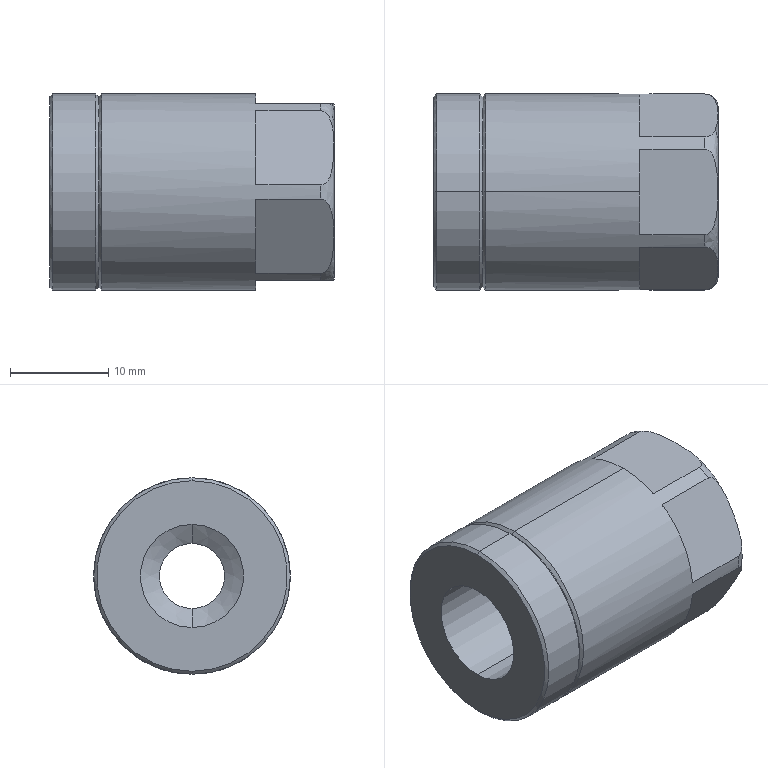Part | STEP file | _20MACJ15010A-Nut | 1 solid | 34 faces | box 29 x 20 x 20 mm | volume 7030 mm3 | plane 14 | cone 10 | cylinder 8 | spline 2 | commonest cylinder face diameters 20 x4 6.647 x2 10.5 x2
STEP:
#1=CARTESIAN_POINT('',(457.,0.,-8.6));
#2=VERTEX_POINT('',#1);
#3=CARTESIAN_POINT('',(457.,0.,8.6));
#4=VERTEX_POINT('',#3);
#5=CARTESIAN_POINT('',(457.,0.,-8.6));
#6=CARTESIAN_POINT('',(457.,-17.2,-8.6));
#7=CARTESIAN_POINT('',(457.,-17.2,8.6));
#8=CARTESIAN_POINT('',(457.,0.,8.6));
#9=(BOUNDED_CURVE()B_SPLINE_CURVE(3,(#5,#6,#7,#8),.UNSPECIFIED.,.F.,.F.)B_SPLINE_CURVE_WITH_KNOTS((4,4),(0.,0.5),.UNSPECIFIED.)CURVE()GEOMETRIC_REPRESENTATION_ITEM()RATIONAL_B_SPLINE_CURVE((1.,0.3333,0.3333,1.))REPRESENTATION_ITEM(''));
#10=EDGE_CURVE('',#2,#4,#9,.T.);
#11=ORIENTED_EDGE('',*,*,#10,.T.);
#12=CARTESIAN_POINT('',(456.942,0.,9.));
#13=VERTEX_POINT('',#12);
#14=CARTESIAN_POINT('',(455.6,0.,8.6));
#15=DIRECTION('',(0.,-1.,0.));
#16=DIRECTION('',(0.,0.,1.));
#17=AXIS2_PLACEMENT_3D('',#14,#15,#16);
#18=CIRCLE('',#17,1.4);
#19=EDGE_CURVE('',#4,#13,#18,.T.);
#20=ORIENTED_EDGE('',*,*,#19,.T.);
#21=CARTESIAN_POINT('',(455.6,-4.359,9.));
#22=VERTEX_POINT('',#21);
#23=CARTESIAN_POINT('',(455.6,-4.359,9.));
#24=CARTESIAN_POINT('',(455.704,-4.359,9.));
#25=CARTESIAN_POINT('',(455.805,-4.332,9.));
#26=CARTESIAN_POINT('',(455.989,-4.239,9.));
#27=CARTESIAN_POINT('',(456.071,-4.174,9.));
#28=CARTESIAN_POINT('',(456.214,-4.029,9.));
#29=CARTESIAN_POINT('',(456.277,-3.947,9.));
#30=CARTESIAN_POINT('',(456.388,-3.775,9.));
#31=CARTESIAN_POINT('',(456.435,-3.685,9.));
#32=CARTESIAN_POINT('',(456.563,-3.407,9.));
#33=CARTESIAN_POINT('',(456.628,-3.211,9.));
#34=CARTESIAN_POINT('',(456.731,-2.819,9.));
#35=CARTESIAN_POINT('',(456.769,-2.621,9.));
#36=CARTESIAN_POINT('',(456.863,-2.023,9.));
#37=CARTESIAN_POINT('',(456.895,-1.62,9.));
#38=CARTESIAN_POINT('',(456.934,-0.8093,9.));
#39=CARTESIAN_POINT('',(456.942,-0.4046,9.));
#40=CARTESIAN_POINT('',(456.942,0.,9.));
#41=B_SPLINE_CURVE_WITH_KNOTS('',3,(#23,#24,#25,#26,#27,#28,#29,#30,#31,#32,#33,#34,#35,#36,#37,#38,#39,#40),.UNSPECIFIED.,.F.,.F.,(4,2,2,2,2,2,2,2,4),(0.,0.0003068,0.0006136,0.0009205,0.001227,0.001841,0.002455,0.003682,0.004909),.UNSPECIFIED.);
#42=EDGE_CURVE('',#22,#13,#41,.T.);
#43=ORIENTED_EDGE('',*,*,#42,.F.);
#44=CARTESIAN_POINT('',(455.6,-5.615,8.275));
#45=VERTEX_POINT('',#44);
#46=CARTESIAN_POINT('',(455.6,0.,0.));
#47=DIRECTION('',(1.,0.,0.));
#48=DIRECTION('',(0.,0.,-1.));
#49=AXIS2_PLACEMENT_3D('',#46,#47,#48);
#50=CIRCLE('',#49,10.);
#51=EDGE_CURVE('',#22,#45,#50,.T.);
#52=ORIENTED_EDGE('',*,*,#51,.T.);
#53=CARTESIAN_POINT('',(455.6,-9.974,0.7251));
#54=VERTEX_POINT('',#53);
#55=CARTESIAN_POINT('',(455.6,-9.974,0.7251));
#56=CARTESIAN_POINT('',(455.704,-9.974,0.7251));
#57=CARTESIAN_POINT('',(455.805,-9.96,0.7487));
#58=CARTESIAN_POINT('',(455.989,-9.914,0.8289));
#59=CARTESIAN_POINT('',(456.071,-9.881,0.885));
#60=CARTESIAN_POINT('',(456.214,-9.809,1.011));
#61=CARTESIAN_POINT('',(456.277,-9.767,1.082));
#62=CARTESIAN_POINT('',(456.388,-9.681,1.231));
#63=CARTESIAN_POINT('',(456.436,-9.636,1.309));
#64=CARTESIAN_POINT('',(456.563,-9.498,1.549));
#65=CARTESIAN_POINT('',(456.628,-9.4,1.719));
#66=CARTESIAN_POINT('',(456.731,-9.204,2.059));
#67=CARTESIAN_POINT('',(456.77,-9.105,2.23));
#68=CARTESIAN_POINT('',(456.863,-8.806,2.748));
#69=CARTESIAN_POINT('',(456.895,-8.604,3.098));
#70=CARTESIAN_POINT('',(456.934,-8.198,3.8));
#71=CARTESIAN_POINT('',(456.942,-7.996,4.151));
#72=CARTESIAN_POINT('',(456.942,-7.591,4.851));
#73=CARTESIAN_POINT('',(456.934,-7.389,5.202));
#74=CARTESIAN_POINT('',(456.895,-6.985,5.902));
#75=CARTESIAN_POINT('',(456.863,-6.783,6.252));
#76=CARTESIAN_POINT('',(456.769,-6.481,6.774));
#77=CARTESIAN_POINT('',(456.729,-6.381,6.947));
#78=CARTESIAN_POINT('',(456.625,-6.184,7.288));
#79=CARTESIAN_POINT('',(456.561,-6.088,7.455));
#80=CARTESIAN_POINT('',(456.391,-5.904,7.774));
#81=CARTESIAN_POINT('',(456.285,-5.815,7.928));
#82=CARTESIAN_POINT('',(456.068,-5.706,8.117));
#83=CARTESIAN_POINT('',(455.988,-5.674,8.172));
#84=CARTESIAN_POINT('',(455.805,-5.628,8.251));
#85=CARTESIAN_POINT('',(455.703,-5.615,8.275));
#86=CARTESIAN_POINT('',(455.6,-5.615,8.275));
#87=B_SPLINE_CURVE_WITH_KNOTS('',3,(#55,#56,#57,#58,#59,#60,#61,#62,#63,#64,#65,#66,#67,#68,#69,#70,#71,#72,#73,#74,#75,#76,#77,#78,#79,#80,#81,#82,#83,#84,#85,#86),.UNSPECIFIED.,.F.,.F.,(4,2,2,2,2,2,2,2,2,2,2,2,2,2,2,4),(0.,0.0003069,0.0006138,0.0009207,0.001228,0.001841,0.002455,0.003683,0.00491,0.006138,0.007365,0.007979,0.008593,0.009207,0.009514,0.009821),.UNSPECIFIED.);
#88=EDGE_CURVE('',#54,#45,#87,.T.);
#89=ORIENTED_EDGE('',*,*,#88,.F.);
#90=CARTESIAN_POINT('',(455.6,-9.974,-0.7251));
#91=VERTEX_POINT('',#90);
#92=CARTESIAN_POINT('',(455.6,0.,0.));
#93=DIRECTION('',(1.,0.,0.));
#94=DIRECTION('',(0.,0.,-1.));
#95=AXIS2_PLACEMENT_3D('',#92,#93,#94);
#96=CIRCLE('',#95,10.);
#97=EDGE_CURVE('',#54,#91,#96,.T.);
#98=ORIENTED_EDGE('',*,*,#97,.T.);
#99=CARTESIAN_POINT('',(455.6,-5.615,-8.275));
#100=VERTEX_POINT('',#99);
#101=CARTESIAN_POINT('',(455.6,-5.615,-8.275));
#102=CARTESIAN_POINT('',(455.704,-5.615,-8.275));
#103=CARTESIAN_POINT('',(455.805,-5.628,-8.251));
#104=CARTESIAN_POINT('',(455.989,-5.675,-8.171));
#105=CARTESIAN_POINT('',(456.071,-5.707,-8.115));
#106=CARTESIAN_POINT('',(456.214,-5.78,-7.989));
#107=CARTESIAN_POINT('',(456.277,-5.821,-7.918));
#108=CARTESIAN_POINT('',(456.388,-5.907,-7.769));
#109=CARTESIAN_POINT('',(456.436,-5.952,-7.691));
#110=CARTESIAN_POINT('',(456.563,-6.091,-7.451));
#111=CARTESIAN_POINT('',(456.628,-6.189,-7.281));
#112=CARTESIAN_POINT('',(456.731,-6.385,-6.941));
#113=CARTESIAN_POINT('',(456.77,-6.484,-6.77));
#114=CARTESIAN_POINT('',(456.863,-6.783,-6.252));
#115=CARTESIAN_POINT('',(456.895,-6.985,-5.902));
#116=CARTESIAN_POINT('',(456.934,-7.39,-5.2));
#117=CARTESIAN_POINT('',(456.942,-7.592,-4.849));
#118=CARTESIAN_POINT('',(456.942,-7.997,-4.149));
#119=CARTESIAN_POINT('',(456.934,-8.199,-3.798));
#120=CARTESIAN_POINT('',(456.895,-8.603,-3.098));
#121=CARTESIAN_POINT('',(456.863,-8.806,-2.748));
#122=CARTESIAN_POINT('',(456.769,-9.107,-2.226));
#123=CARTESIAN_POINT('',(456.729,-9.207,-2.053));
#124=CARTESIAN_POINT('',(456.625,-9.404,-1.712));
#125=CARTESIAN_POINT('',(456.561,-9.501,-1.545));
#126=CARTESIAN_POINT('',(456.391,-9.684,-1.226));
#127=CARTESIAN_POINT('',(456.285,-9.773,-1.072));
#128=CARTESIAN_POINT('',(456.068,-9.883,-0.8826));
#129=CARTESIAN_POINT('',(455.988,-9.914,-0.8285));
#130=CARTESIAN_POINT('',(455.805,-9.96,-0.7485));
#131=CARTESIAN_POINT('',(455.703,-9.974,-0.7251));
#132=CARTESIAN_POINT('',(455.6,-9.974,-0.7251));
#133=B_SPLINE_CURVE_WITH_KNOTS('',3,(#101,#102,#103,#104,#105,#106,#107,#108,#109,#110,#111,#112,#113,#114,#115,#116,#117,#118,#119,#120,#121,#122,#123,#124,#125,#126,#127,#128,#129,#130,#131,#132),.UNSPECIFIED.,.F.,.F.,(4,2,2,2,2,2,2,2,2,2,2,2,2,2,2,4),(0.,0.0003069,0.0006138,0.0009207,0.001228,0.001841,0.002455,0.003683,0.00491,0.006138,0.007365,0.007979,0.008593,0.009207,0.009514,0.009821),.UNSPECIFIED.);
#134=EDGE_CURVE('',#100,#91,#133,.T.);
#135=ORIENTED_EDGE('',*,*,#134,.F.);
#136=CARTESIAN_POINT('',(455.6,-4.359,-9.));
#137=VERTEX_POINT('',#136);
#138=CARTESIAN_POINT('',(455.6,0.,0.));
#139=DIRECTION('',(1.,0.,0.));
#140=DIRECTION('',(0.,0.,-1.));
#141=AXIS2_PLACEMENT_3D('',#138,#139,#140);
#142=CIRCLE('',#141,10.);
#143=EDGE_CURVE('',#100,#137,#142,.T.);
#144=ORIENTED_EDGE('',*,*,#143,.T.);
#145=CARTESIAN_POINT('',(456.942,0.,-9.));
#146=VERTEX_POINT('',#145);
#147=CARTESIAN_POINT('',(456.942,0.,-9.));
#148=CARTESIAN_POINT('',(456.942,-0.4048,-9.));
#149=CARTESIAN_POINT('',(456.934,-0.8093,-9.));
#150=CARTESIAN_POINT('',(456.895,-1.618,-9.));
#151=CARTESIAN_POINT('',(456.863,-2.022,-9.));
#152=CARTESIAN_POINT('',(456.769,-2.626,-9.));
#153=CARTESIAN_POINT('',(456.729,-2.825,-9.));
#154=CARTESIAN_POINT('',(456.625,-3.219,-9.));
#155=CARTESIAN_POINT('',(456.561,-3.412,-9.));
#156=CARTESIAN_POINT('',(456.391,-3.78,-9.));
#157=CARTESIAN_POINT('',(456.285,-3.958,-9.));
#158=CARTESIAN_POINT('',(456.068,-4.177,-9.));
#159=CARTESIAN_POINT('',(455.988,-4.239,-9.));
#160=CARTESIAN_POINT('',(455.805,-4.332,-9.));
#161=CARTESIAN_POINT('',(455.703,-4.359,-9.));
#162=CARTESIAN_POINT('',(455.6,-4.359,-9.));
#163=B_SPLINE_CURVE_WITH_KNOTS('',3,(#147,#148,#149,#150,#151,#152,#153,#154,#155,#156,#157,#158,#159,#160,#161,#162),.UNSPECIFIED.,.F.,.F.,(4,2,2,2,2,2,2,4),(0.004909,0.006137,0.007365,0.007979,0.008593,0.009207,0.009514,0.009821),.UNSPECIFIED.);
#164=EDGE_CURVE('',#146,#137,#163,.T.);
#165=ORIENTED_EDGE('',*,*,#164,.F.);
#166=CARTESIAN_POINT('',(455.6,0.,-8.6));
#167=DIRECTION('',(0.,1.,0.));
#168=DIRECTION('',(0.,0.,-1.));
#169=AXIS2_PLACEMENT_3D('',#166,#167,#168);
#170=CIRCLE('',#169,1.4);
#171=EDGE_CURVE('',#2,#146,#170,.T.);
#172=ORIENTED_EDGE('',*,*,#171,.F.);
#173=EDGE_LOOP('',(#11,#20,#43,#52,#89,#98,#135,#144,#165,#172));
#174=FACE_OUTER_BOUND('',#173,.T.);
#175=CARTESIAN_POINT('',(457.,0.,8.6));
#176=CARTESIAN_POINT('',(457.,-17.2,8.6));
#177=CARTESIAN_POINT('',(457.,-17.2,-8.6));
#178=CARTESIAN_POINT('',(457.,0.,-8.6));
#179=CARTESIAN_POINT('',(457.,0.,9.42));
#180=CARTESIAN_POINT('',(457.,-18.84,9.42));
#181=CARTESIAN_POINT('',(457.,-18.84,-9.42));
#182=CARTESIAN_POINT('',(457.,0.,-9.42));
#183=CARTESIAN_POINT('',(456.42,0.,10.));
#184=CARTESIAN_POINT('',(456.42,-20.,10.));
#185=CARTESIAN_POINT('',(456.42,-20.,-10.));
#186=CARTESIAN_POINT('',(456.42,0.,-10.));
#187=CARTESIAN_POINT('',(455.6,0.,10.));
#188=CARTESIAN_POINT('',(455.6,-20.,10.));
#189=CARTESIAN_POINT('',(455.6,-20.,-10.));
#190=CARTESIAN_POINT('',(455.6,0.,-10.));
#191=(BOUNDED_SURFACE()B_SPLINE_SURFACE(3,3,((#175,#176,#177,#178),(#179,#180,#181,#182),(#183,#184,#185,#186),(#187,#188,#189,#190)),.UNSPECIFIED.,.F.,.F.,.T.)B_SPLINE_SURFACE_WITH_KNOTS((4,4),(4,4),(0.,1.),(0.,1.),.UNSPECIFIED.)GEOMETRIC_REPRESENTATION_ITEM()RATIONAL_B_SPLINE_SURFACE(((1.,0.3333,0.3333,1.),(0.8047,0.2682,0.2682,0.8047),(0.8047,0.2682,0.2682,0.8047),(1.,0.3333,0.3333,1.)))REPRESENTATION_ITEM('')SURFACE());
#192=ADVANCED_FACE('',(#174),#191,.T.);
#193=CARTESIAN_POINT('',(449.,4.359,-9.));
#194=VERTEX_POINT('',#193);
#195=CARTESIAN_POINT('',(449.,0.,-10.));
#196=VERTEX_POINT('',#195);
#197=CARTESIAN_POINT('',(449.,0.,0.));
#198=DIRECTION('',(-1.,0.,0.));
#199=DIRECTION('',(0.,0.,1.));
#200=AXIS2_PLACEMENT_3D('',#197,#198,#199);
#201=CIRCLE('',#200,10.);
#202=EDGE_CURVE('',#194,#196,#201,.T.);
#203=ORIENTED_EDGE('',*,*,#202,.T.);
#204=CARTESIAN_POINT('',(433.3,0.,-10.));
#205=VERTEX_POINT('',#204);
#206=CARTESIAN_POINT('',(457.,0.,-10.));
#207=DIRECTION('',(-1.,0.,0.));
#208=VECTOR('',#207,1000.);
#209=LINE('',#206,#208);
#210=EDGE_CURVE('',#196,#205,#209,.T.);
#211=ORIENTED_EDGE('',*,*,#210,.T.);
#212=CARTESIAN_POINT('',(433.3,0.,10.));
#213=VERTEX_POINT('',#212);
#214=CARTESIAN_POINT('',(433.3,0.,0.));
#215=DIRECTION('',(1.,0.,0.));
#216=DIRECTION('',(0.,0.,1.));
#217=AXIS2_PLACEMENT_3D('',#214,#215,#216);
#218=CIRCLE('',#217,10.);
#219=EDGE_CURVE('',#205,#213,#218,.T.);
#220=ORIENTED_EDGE('',*,*,#219,.T.);
#221=CARTESIAN_POINT('',(449.,0.,10.));
#222=VERTEX_POINT('',#221);
#223=CARTESIAN_POINT('',(457.,0.,10.));
#224=DIRECTION('',(-1.,0.,0.));
#225=VECTOR('',#224,1000.);
#226=LINE('',#223,#225);
#227=EDGE_CURVE('',#222,#213,#226,.T.);
#228=ORIENTED_EDGE('',*,*,#227,.F.);
#229=CARTESIAN_POINT('',(449.,4.359,9.));
#230=VERTEX_POINT('',#229);
#231=CARTESIAN_POINT('',(449.,0.,0.));
#232=DIRECTION('',(-1.,0.,0.));
#233=DIRECTION('',(0.,0.,1.));
#234=AXIS2_PLACEMENT_3D('',#231,#232,#233);
#235=CIRCLE('',#234,10.);
#236=EDGE_CURVE('',#222,#230,#235,.T.);
#237=ORIENTED_EDGE('',*,*,#236,.T.);
#238=CARTESIAN_POINT('',(455.6,4.359,9.));
#239=VERTEX_POINT('',#238);
#240=CARTESIAN_POINT('',(457.,4.359,9.));
#241=DIRECTION('',(1.,0.,0.));
#242=VECTOR('',#241,1000.);
#243=LINE('',#240,#242);
#244=EDGE_CURVE('',#230,#239,#243,.T.);
#245=ORIENTED_EDGE('',*,*,#244,.T.);
#246=CARTESIAN_POINT('',(455.6,5.615,8.275));
#247=VERTEX_POINT('',#246);
#248=CARTESIAN_POINT('',(455.6,0.,0.));
#249=DIRECTION('',(1.,0.,0.));
#250=DIRECTION('',(0.,0.,-1.));
#251=AXIS2_PLACEMENT_3D('',#248,#249,#250);
#252=CIRCLE('',#251,10.);
#253=EDGE_CURVE('',#247,#239,#252,.T.);
#254=ORIENTED_EDGE('',*,*,#253,.F.);
#255=CARTESIAN_POINT('',(449.,5.615,8.275));
#256=VERTEX_POINT('',#255);
#257=CARTESIAN_POINT('',(457.,5.615,8.275));
#258=DIRECTION('',(-1.,0.,0.));
#259=VECTOR('',#258,1000.);
#260=LINE('',#257,#259);
#261=EDGE_CURVE('',#247,#256,#260,.T.);
#262=ORIENTED_EDGE('',*,*,#261,.T.);
#263=CARTESIAN_POINT('',(449.,9.974,0.7251));
#264=VERTEX_POINT('',#263);
#265=CARTESIAN_POINT('',(449.,0.,0.));
#266=DIRECTION('',(-1.,0.,0.));
#267=DIRECTION('',(0.,0.,1.));
#268=AXIS2_PLACEMENT_3D('',#265,#266,#267);
#269=CIRCLE('',#268,10.);
#270=EDGE_CURVE('',#256,#264,#269,.T.);
#271=ORIENTED_EDGE('',*,*,#270,.T.);
#272=CARTESIAN_POINT('',(455.6,9.974,0.7251));
#273=VERTEX_POINT('',#272);
#274=CARTESIAN_POINT('',(457.,9.974,0.7251));
#275=DIRECTION('',(1.,0.,0.));
#276=VECTOR('',#275,1000.);
#277=LINE('',#274,#276);
#278=EDGE_CURVE('',#264,#273,#277,.T.);
#279=ORIENTED_EDGE('',*,*,#278,.T.);
#280=CARTESIAN_POINT('',(455.6,9.974,-0.7251));
#281=VERTEX_POINT('',#280);
#282=CARTESIAN_POINT('',(455.6,0.,0.));
#283=DIRECTION('',(1.,0.,0.));
#284=DIRECTION('',(0.,0.,-1.));
#285=AXIS2_PLACEMENT_3D('',#282,#283,#284);
#286=CIRCLE('',#285,10.);
#287=EDGE_CURVE('',#281,#273,#286,.T.);
#288=ORIENTED_EDGE('',*,*,#287,.F.);
#289=CARTESIAN_POINT('',(449.,9.974,-0.7251));
#290=VERTEX_POINT('',#289);
#291=CARTESIAN_POINT('',(457.,9.974,-0.7251));
#292=DIRECTION('',(-1.,0.,0.));
#293=VECTOR('',#292,1000.);
#294=LINE('',#291,#293);
#295=EDGE_CURVE('',#281,#290,#294,.T.);
#296=ORIENTED_EDGE('',*,*,#295,.T.);
#297=CARTESIAN_POINT('',(449.,5.615,-8.275));
#298=VERTEX_POINT('',#297);
#299=CARTESIAN_POINT('',(449.,0.,0.));
#300=DIRECTION('',(-1.,0.,0.));
#301=DIRECTION('',(0.,0.,1.));
#302=AXIS2_PLACEMENT_3D('',#299,#300,#301);
#303=CIRCLE('',#302,10.);
#304=EDGE_CURVE('',#290,#298,#303,.T.);
#305=ORIENTED_EDGE('',*,*,#304,.T.);
#306=CARTESIAN_POINT('',(455.6,5.615,-8.275));
#307=VERTEX_POINT('',#306);
#308=CARTESIAN_POINT('',(457.,5.615,-8.275));
#309=DIRECTION('',(1.,0.,0.));
#310=VECTOR('',#309,1000.);
#311=LINE('',#308,#310);
#312=EDGE_CURVE('',#298,#307,#311,.T.);
#313=ORIENTED_EDGE('',*,*,#312,.T.);
#314=CARTESIAN_POINT('',(455.6,4.359,-9.));
#315=VERTEX_POINT('',#314);
#316=CARTESIAN_POINT('',(455.6,0.,0.));
#317=DIRECTION('',(1.,0.,0.));
#318=DIRECTION('',(0.,0.,-1.));
#319=AXIS2_PLACEMENT_3D('',#316,#317,#318);
#320=CIRCLE('',#319,10.);
#321=EDGE_CURVE('',#315,#307,#320,.T.);
#322=ORIENTED_EDGE('',*,*,#321,.F.);
#323=CARTESIAN_POINT('',(457.,4.359,-9.));
#324=DIRECTION('',(-1.,0.,0.));
#325=VECTOR('',#324,1000.);
#326=LINE('',#323,#325);
#327=EDGE_CURVE('',#315,#194,#326,.T.);
#328=ORIENTED_EDGE('',*,*,#327,.T.);
#329=EDGE_LOOP('',(#203,#211,#220,#228,#237,#245,#254,#262,#271,#279,#288,#296,#305,#313,#322,#328));
#330=FACE_OUTER_BOUND('',#329,.T.);
#331=CARTESIAN_POINT('',(457.,0.,0.));
#332=DIRECTION('',(-1.,0.,0.));
#333=DIRECTION('',(0.,0.,1.));
#334=AXIS2_PLACEMENT_3D('',#331,#332,#333);
#335=CYLINDRICAL_SURFACE('',#334,10.);
#336=ADVANCED_FACE('',(#330),#335,.T.);
#337=CARTESIAN_POINT('',(433.,0.,-9.7));
#338=VERTEX_POINT('',#337);
#339=CARTESIAN_POINT('',(433.,0.,9.7));
#340=VERTEX_POINT('',#339);
#341=CARTESIAN_POINT('',(433.,0.,0.));
#342=DIRECTION('',(1.,0.,0.));
#343=DIRECTION('',(0.,0.,-1.));
#344=AXIS2_PLACEMENT_3D('',#341,#342,#343);
#345=CIRCLE('',#344,9.7);
#346=EDGE_CURVE('',#338,#340,#345,.T.);
#347=ORIENTED_EDGE('',*,*,#346,.T.);
#348=CARTESIAN_POINT('',(433.3,0.,10.));
#349=DIRECTION('',(0.7071,0.,0.7071));
#350=VECTOR('',#349,1000.);
#351=LINE('',#348,#350);
#352=EDGE_CURVE('',#340,#213,#351,.T.);
#353=ORIENTED_EDGE('',*,*,#352,.T.);
#354=ORIENTED_EDGE('',*,*,#219,.F.);
#355=CARTESIAN_POINT('',(433.3,0.,-10.));
#356=DIRECTION('',(0.7071,0.,-0.7071));
#357=VECTOR('',#356,1000.);
#358=LINE('',#355,#357);
#359=EDGE_CURVE('',#338,#205,#358,.T.);
#360=ORIENTED_EDGE('',*,*,#359,.F.);
#361=EDGE_LOOP('',(#347,#353,#354,#360));
#362=FACE_OUTER_BOUND('',#361,.T.);
#363=CARTESIAN_POINT('',(433.3,0.,0.));
#364=DIRECTION('',(1.,0.,0.));
#365=DIRECTION('',(0.,0.,-1.));
#366=AXIS2_PLACEMENT_3D('',#363,#364,#365);
#367=CONICAL_SURFACE('',#366,10.,0.7854);
#368=ADVANCED_FACE('',(#362),#367,.T.);
#369=ORIENTED_EDGE('',*,*,#346,.F.);
#370=CARTESIAN_POINT('',(432.7,0.,-10.));
#371=VERTEX_POINT('',#370);
#372=CARTESIAN_POINT('',(432.7,0.,-10.));
#373=DIRECTION('',(-0.7071,0.,-0.7071));
#374=VECTOR('',#373,1000.);
#375=LINE('',#372,#374);
#376=EDGE_CURVE('',#338,#371,#375,.T.);
#377=ORIENTED_EDGE('',*,*,#376,.T.);
#378=CARTESIAN_POINT('',(432.7,0.,10.));
#379=VERTEX_POINT('',#378);
#380=CARTESIAN_POINT('',(432.7,0.,0.));
#381=DIRECTION('',(1.,0.,0.));
#382=DIRECTION('',(0.,0.,1.));
#383=AXIS2_PLACEMENT_3D('',#380,#381,#382);
#384=CIRCLE('',#383,10.);
#385=EDGE_CURVE('',#371,#379,#384,.T.);
#386=ORIENTED_EDGE('',*,*,#385,.T.);
#387=CARTESIAN_POINT('',(432.7,0.,10.));
#388=DIRECTION('',(-0.7071,0.,0.7071));
#389=VECTOR('',#388,1000.);
#390=LINE('',#387,#389);
#391=EDGE_CURVE('',#340,#379,#390,.T.);
#392=ORIENTED_EDGE('',*,*,#391,.F.);
#393=EDGE_LOOP('',(#369,#377,#386,#392));
#394=FACE_OUTER_BOUND('',#393,.T.);
#395=CARTESIAN_POINT('',(432.7,0.,0.));
#396=DIRECTION('',(-1.,0.,0.));
#397=DIRECTION('',(0.,0.,1.));
#398=AXIS2_PLACEMENT_3D('',#395,#396,#397);
#399=CONICAL_SURFACE('',#398,10.,0.7854);
#400=ADVANCED_FACE('',(#394),#399,.T.);
#401=ORIENTED_EDGE('',*,*,#385,.F.);
#402=CARTESIAN_POINT('',(428.3,0.,-10.));
#403=VERTEX_POINT('',#402);
#404=CARTESIAN_POINT('',(457.,0.,-10.));
#405=DIRECTION('',(-1.,0.,0.));
#406=VECTOR('',#405,1000.);
#407=LINE('',#404,#406);
#408=EDGE_CURVE('',#371,#403,#407,.T.);
#409=ORIENTED_EDGE('',*,*,#408,.T.);
#410=CARTESIAN_POINT('',(428.3,0.,10.));
#411=VERTEX_POINT('',#410);
#412=CARTESIAN_POINT('',(428.3,0.,0.));
#413=DIRECTION('',(1.,0.,0.));
#414=DIRECTION('',(0.,0.,1.));
#415=AXIS2_PLACEMENT_3D('',#412,#413,#414);
#416=CIRCLE('',#415,10.);
#417=EDGE_CURVE('',#403,#411,#416,.T.);
#418=ORIENTED_EDGE('',*,*,#417,.T.);
#419=CARTESIAN_POINT('',(457.,0.,10.));
#420=DIRECTION('',(-1.,0.,0.));
#421=VECTOR('',#420,1000.);
#422=LINE('',#419,#421);
#423=EDGE_CURVE('',#379,#411,#422,.T.);
#424=ORIENTED_EDGE('',*,*,#423,.F.);
#425=EDGE_LOOP('',(#401,#409,#418,#424));
#426=FACE_OUTER_BOUND('',#425,.T.);
#427=CARTESIAN_POINT('',(457.,0.,0.));
#428=DIRECTION('',(-1.,0.,0.));
#429=DIRECTION('',(0.,0.,1.));
#430=AXIS2_PLACEMENT_3D('',#427,#428,#429);
#431=CYLINDRICAL_SURFACE('',#430,10.);
#432=ADVANCED_FACE('',(#426),#431,.T.);
#433=CARTESIAN_POINT('',(428.,0.,-9.7));
#434=VERTEX_POINT('',#433);
#435=CARTESIAN_POINT('',(428.,0.,9.7));
#436=VERTEX_POINT('',#435);
#437=CARTESIAN_POINT('',(428.,0.,0.));
#438=DIRECTION('',(1.,0.,0.));
#439=DIRECTION('',(0.,0.,-1.));
#440=AXIS2_PLACEMENT_3D('',#437,#438,#439);
#441=CIRCLE('',#440,9.7);
#442=EDGE_CURVE('',#434,#436,#441,.T.);
#443=ORIENTED_EDGE('',*,*,#442,.T.);
#444=CARTESIAN_POINT('',(428.3,0.,10.));
#445=DIRECTION('',(0.7071,0.,0.7071));
#446=VECTOR('',#445,1000.);
#447=LINE('',#444,#446);
#448=EDGE_CURVE('',#436,#411,#447,.T.);
#449=ORIENTED_EDGE('',*,*,#448,.T.);
#450=ORIENTED_EDGE('',*,*,#417,.F.);
#451=CARTESIAN_POINT('',(428.3,0.,-10.));
#452=DIRECTION('',(0.7071,0.,-0.7071));
#453=VECTOR('',#452,1000.);
#454=LINE('',#451,#453);
#455=EDGE_CURVE('',#434,#403,#454,.T.);
#456=ORIENTED_EDGE('',*,*,#455,.F.);
#457=EDGE_LOOP('',(#443,#449,#450,#456));
#458=FACE_OUTER_BOUND('',#457,.T.);
#459=CARTESIAN_POINT('',(428.3,0.,0.));
#460=DIRECTION('',(1.,0.,0.));
#461=DIRECTION('',(0.,0.,-1.));
#462=AXIS2_PLACEMENT_3D('',#459,#460,#461);
#463=CONICAL_SURFACE('',#462,10.,0.7854);
#464=ADVANCED_FACE('',(#458),#463,.T.);
#465=CARTESIAN_POINT('',(456.323,-3.323,0.));
#466=VERTEX_POINT('',#465);
#467=CARTESIAN_POINT('',(456.323,0.,-3.323));
#468=VERTEX_POINT('',#467);
#469=CARTESIAN_POINT('',(456.323,0.,0.));
#470=DIRECTION('',(1.,0.,0.));
#471=DIRECTION('',(0.,0.,-1.));
#472=AXIS2_PLACEMENT_3D('',#469,#470,#471);
#473=CIRCLE('',#472,3.323);
#474=EDGE_CURVE('',#466,#468,#473,.T.);
#475=ORIENTED_EDGE('',*,*,#474,.F.);
#476=CARTESIAN_POINT('',(457.,-4.,0.));
#477=VERTEX_POINT('',#476);
#478=CARTESIAN_POINT('',(457.,-4.,0.));
#479=DIRECTION('',(0.7071,-0.7071,0.));
#480=VECTOR('',#479,1000.);
#481=LINE('',#478,#480);
#482=EDGE_CURVE('',#466,#477,#481,.T.);
#483=ORIENTED_EDGE('',*,*,#482,.T.);
#484=CARTESIAN_POINT('',(457.,4.,0.));
#485=VERTEX_POINT('',#484);
#486=CARTESIAN_POINT('',(457.,0.,0.));
#487=DIRECTION('',(1.,0.,0.));
#488=DIRECTION('',(0.,1.,0.));
#489=AXIS2_PLACEMENT_3D('',#486,#487,#488);
#490=CIRCLE('',#489,4.);
#491=EDGE_CURVE('',#477,#485,#490,.T.);
#492=ORIENTED_EDGE('',*,*,#491,.T.);
#493=CARTESIAN_POINT('',(456.323,3.323,0.));
#494=VERTEX_POINT('',#493);
#495=CARTESIAN_POINT('',(457.,4.,0.));
#496=DIRECTION('',(0.7071,0.7071,0.));
#497=VECTOR('',#496,1000.);
#498=LINE('',#495,#497);
#499=EDGE_CURVE('',#494,#485,#498,.T.);
#500=ORIENTED_EDGE('',*,*,#499,.F.);
#501=CARTESIAN_POINT('',(456.323,0.,0.));
#502=DIRECTION('',(1.,0.,0.));
#503=DIRECTION('',(0.,0.,-1.));
#504=AXIS2_PLACEMENT_3D('',#501,#502,#503);
#505=CIRCLE('',#504,3.323);
#506=EDGE_CURVE('',#468,#494,#505,.T.);
#507=ORIENTED_EDGE('',*,*,#506,.F.);
#508=EDGE_LOOP('',(#475,#483,#492,#500,#507));
#509=FACE_OUTER_BOUND('',#508,.T.);
#510=CARTESIAN_POINT('',(457.,0.,0.));
#511=DIRECTION('',(1.,0.,0.));
#512=DIRECTION('',(0.,1.,0.));
#513=AXIS2_PLACEMENT_3D('',#510,#511,#512);
#514=CONICAL_SURFACE('',#513,4.,0.7854);
#515=ADVANCED_FACE('',(#509),#514,.F.);
#516=CARTESIAN_POINT('',(456.323,0.,3.323));
#517=VERTEX_POINT('',#516);
#518=CARTESIAN_POINT('',(456.323,0.,0.));
#519=DIRECTION('',(1.,0.,0.));
#520=DIRECTION('',(0.,0.,-1.));
#521=AXIS2_PLACEMENT_3D('',#518,#519,#520);
#522=CIRCLE('',#521,3.323);
#523=EDGE_CURVE('',#517,#466,#522,.T.);
#524=ORIENTED_EDGE('',*,*,#523,.T.);
#525=ORIENTED_EDGE('',*,*,#474,.T.);
#526=CARTESIAN_POINT('',(443.462,0.,-3.324));
#527=VERTEX_POINT('',#526);
#528=CARTESIAN_POINT('',(457.,0.,-3.324));
#529=DIRECTION('',(-1.,0.,0.));
#530=VECTOR('',#529,1000.);
#531=LINE('',#528,#530);
#532=EDGE_CURVE('',#468,#527,#531,.T.);
#533=ORIENTED_EDGE('',*,*,#532,.T.);
#534=CARTESIAN_POINT('',(443.462,0.,3.324));
#535=VERTEX_POINT('',#534);
#536=CARTESIAN_POINT('',(443.462,0.,0.));
#537=DIRECTION('',(1.,0.,0.));
#538=DIRECTION('',(0.,0.,1.));
#539=AXIS2_PLACEMENT_3D('',#536,#537,#538);
#540=CIRCLE('',#539,3.324);
#541=EDGE_CURVE('',#535,#527,#540,.T.);
#542=ORIENTED_EDGE('',*,*,#541,.F.);
#543=CARTESIAN_POINT('',(457.,0.,3.324));
#544=DIRECTION('',(-1.,0.,0.));
#545=VECTOR('',#544,1000.);
#546=LINE('',#543,#545);
#547=EDGE_CURVE('',#517,#535,#546,.T.);
#548=ORIENTED_EDGE('',*,*,#547,.F.);
#549=EDGE_LOOP('',(#524,#525,#533,#542,#548));
#550=FACE_OUTER_BOUND('',#549,.T.);
#551=CARTESIAN_POINT('',(457.,0.,0.));
#552=DIRECTION('',(-1.,0.,0.));
#553=DIRECTION('',(0.,0.,1.));
#554=AXIS2_PLACEMENT_3D('',#551,#552,#553);
#555=CYLINDRICAL_SURFACE('',#554,3.324);
#556=ADVANCED_FACE('',(#550),#555,.F.);
#557=CARTESIAN_POINT('',(442.35,0.,-5.25));
#558=VERTEX_POINT('',#557);
#559=CARTESIAN_POINT('',(442.35,0.,5.25));
#560=VERTEX_POINT('',#559);
#561=CARTESIAN_POINT('',(442.35,0.,0.));
#562=DIRECTION('',(-1.,0.,0.));
#563=DIRECTION('',(0.,0.,1.));
#564=AXIS2_PLACEMENT_3D('',#561,#562,#563);
#565=CIRCLE('',#564,5.25);
#566=EDGE_CURVE('',#558,#560,#565,.T.);
#567=ORIENTED_EDGE('',*,*,#566,.F.);
#568=CARTESIAN_POINT('',(428.,0.,-5.25));
#569=VERTEX_POINT('',#568);
#570=CARTESIAN_POINT('',(457.,0.,-5.25));
#571=DIRECTION('',(-1.,0.,0.));
#572=VECTOR('',#571,1000.);
#573=LINE('',#570,#572);
#574=EDGE_CURVE('',#558,#569,#573,.T.);
#575=ORIENTED_EDGE('',*,*,#574,.T.);
#576=CARTESIAN_POINT('',(428.,0.,5.25));
#577=VERTEX_POINT('',#576);
#578=CARTESIAN_POINT('',(428.,0.,0.));
#579=DIRECTION('',(-1.,0.,0.));
#580=DIRECTION('',(0.,0.,1.));
#581=AXIS2_PLACEMENT_3D('',#578,#579,#580);
#582=CIRCLE('',#581,5.25);
#583=EDGE_CURVE('',#569,#577,#582,.T.);
#584=ORIENTED_EDGE('',*,*,#583,.T.);
#585=CARTESIAN_POINT('',(457.,0.,5.25));
#586=DIRECTION('',(-1.,0.,0.));
#587=VECTOR('',#586,1000.);
#588=LINE('',#585,#587);
#589=EDGE_CURVE('',#560,#577,#588,.T.);
#590=ORIENTED_EDGE('',*,*,#589,.F.);
#591=EDGE_LOOP('',(#567,#575,#584,#590));
#592=FACE_OUTER_BOUND('',#591,.T.);
#593=CARTESIAN_POINT('',(457.,0.,0.));
#594=DIRECTION('',(-1.,0.,0.));
#595=DIRECTION('',(0.,0.,1.));
#596=AXIS2_PLACEMENT_3D('',#593,#594,#595);
#597=CYLINDRICAL_SURFACE('',#596,5.25);
#598=ADVANCED_FACE('',(#592),#597,.F.);
#599=ORIENTED_EDGE('',*,*,#541,.T.);
#600=CARTESIAN_POINT('',(442.35,0.,-5.25));
#601=DIRECTION('',(-0.5,0.,-0.866));
#602=VECTOR('',#601,1000.);
#603=LINE('',#600,#602);
#604=EDGE_CURVE('',#527,#558,#603,.T.);
#605=ORIENTED_EDGE('',*,*,#604,.T.);
#606=ORIENTED_EDGE('',*,*,#566,.T.);
#607=CARTESIAN_POINT('',(442.35,0.,5.25));
#608=DIRECTION('',(-0.5,0.,0.866));
#609=VECTOR('',#608,1000.);
#610=LINE('',#607,#609);
#611=EDGE_CURVE('',#535,#560,#610,.T.);
#612=ORIENTED_EDGE('',*,*,#611,.F.);
#613=EDGE_LOOP('',(#599,#605,#606,#612));
#614=FACE_OUTER_BOUND('',#613,.T.);
#615=CARTESIAN_POINT('',(442.35,0.,0.));
#616=DIRECTION('',(-1.,0.,0.));
#617=DIRECTION('',(0.,0.,1.));
#618=AXIS2_PLACEMENT_3D('',#615,#616,#617);
#619=CONICAL_SURFACE('',#618,5.25,1.047);
#620=ADVANCED_FACE('',(#614),#619,.F.);
#621=ORIENTED_EDGE('',*,*,#210,.F.);
#622=CARTESIAN_POINT('',(449.,-4.359,-9.));
#623=VERTEX_POINT('',#622);
#624=CARTESIAN_POINT('',(449.,0.,0.));
#625=DIRECTION('',(-1.,0.,0.));
#626=DIRECTION('',(0.,0.,1.));
#627=AXIS2_PLACEMENT_3D('',#624,#625,#626);
#628=CIRCLE('',#627,10.);
#629=EDGE_CURVE('',#196,#623,#628,.T.);
#630=ORIENTED_EDGE('',*,*,#629,.T.);
#631=CARTESIAN_POINT('',(457.,-4.359,-9.));
#632=DIRECTION('',(1.,0.,0.));
#633=VECTOR('',#632,1000.);
#634=LINE('',#631,#633);
#635=EDGE_CURVE('',#623,#137,#634,.T.);
#636=ORIENTED_EDGE('',*,*,#635,.T.);
#637=ORIENTED_EDGE('',*,*,#143,.F.);
#638=CARTESIAN_POINT('',(449.,-5.615,-8.275));
#639=VERTEX_POINT('',#638);
#640=CARTESIAN_POINT('',(457.,-5.615,-8.275));
#641=DIRECTION('',(-1.,0.,0.));
#642=VECTOR('',#641,1000.);
#643=LINE('',#640,#642);
#644=EDGE_CURVE('',#100,#639,#643,.T.);
#645=ORIENTED_EDGE('',*,*,#644,.T.);
#646=CARTESIAN_POINT('',(449.,-9.974,-0.7251));
#647=VERTEX_POINT('',#646);
#648=CARTESIAN_POINT('',(449.,0.,0.));
#649=DIRECTION('',(-1.,0.,0.));
#650=DIRECTION('',(0.,0.,1.));
#651=AXIS2_PLACEMENT_3D('',#648,#649,#650);
#652=CIRCLE('',#651,10.);
#653=EDGE_CURVE('',#639,#647,#652,.T.);
#654=ORIENTED_EDGE('',*,*,#653,.T.);
#655=CARTESIAN_POINT('',(457.,-9.974,-0.7251));
#656=DIRECTION('',(1.,0.,0.));
#657=VECTOR('',#656,1000.);
#658=LINE('',#655,#657);
#659=EDGE_CURVE('',#647,#91,#658,.T.);
#660=ORIENTED_EDGE('',*,*,#659,.T.);
#661=ORIENTED_EDGE('',*,*,#97,.F.);
#662=CARTESIAN_POINT('',(449.,-9.974,0.7251));
#663=VERTEX_POINT('',#662);
#664=CARTESIAN_POINT('',(457.,-9.974,0.7251));
#665=DIRECTION('',(-1.,0.,0.));
#666=VECTOR('',#665,1000.);
#667=LINE('',#664,#666);
#668=EDGE_CURVE('',#54,#663,#667,.T.);
#669=ORIENTED_EDGE('',*,*,#668,.T.);
#670=CARTESIAN_POINT('',(449.,-5.615,8.275));
#671=VERTEX_POINT('',#670);
#672=CARTESIAN_POINT('',(449.,0.,0.));
#673=DIRECTION('',(-1.,0.,0.));
#674=DIRECTION('',(0.,0.,1.));
#675=AXIS2_PLACEMENT_3D('',#672,#673,#674);
#676=CIRCLE('',#675,10.);
#677=EDGE_CURVE('',#663,#671,#676,.T.);
#678=ORIENTED_EDGE('',*,*,#677,.T.);
#679=CARTESIAN_POINT('',(457.,-5.615,8.275));
#680=DIRECTION('',(1.,0.,0.));
#681=VECTOR('',#680,1000.);
#682=LINE('',#679,#681);
#683=EDGE_CURVE('',#671,#45,#682,.T.);
#684=ORIENTED_EDGE('',*,*,#683,.T.);
#685=ORIENTED_EDGE('',*,*,#51,.F.);
#686=CARTESIAN_POINT('',(449.,-4.359,9.));
#687=VERTEX_POINT('',#686);
#688=CARTESIAN_POINT('',(457.,-4.359,9.));
#689=DIRECTION('',(-1.,0.,0.));
#690=VECTOR('',#689,1000.);
#691=LINE('',#688,#690);
#692=EDGE_CURVE('',#22,#687,#691,.T.);
#693=ORIENTED_EDGE('',*,*,#692,.T.);
#694=CARTESIAN_POINT('',(449.,0.,0.));
#695=DIRECTION('',(-1.,0.,0.));
#696=DIRECTION('',(0.,0.,1.));
#697=AXIS2_PLACEMENT_3D('',#694,#695,#696);
#698=CIRCLE('',#697,10.);
#699=EDGE_CURVE('',#687,#222,#698,.T.);
#700=ORIENTED_EDGE('',*,*,#699,.T.);
#701=ORIENTED_EDGE('',*,*,#227,.T.);
#702=CARTESIAN_POINT('',(433.3,0.,0.));
#703=DIRECTION('',(1.,0.,0.));
#704=DIRECTION('',(0.,0.,1.));
#705=AXIS2_PLACEMENT_3D('',#702,#703,#704);
#706=CIRCLE('',#705,10.);
#707=EDGE_CURVE('',#213,#205,#706,.T.);
#708=ORIENTED_EDGE('',*,*,#707,.T.);
#709=EDGE_LOOP('',(#621,#630,#636,#637,#645,#654,#660,#661,#669,#678,#684,#685,#693,#700,#701,#708));
#710=FACE_OUTER_BOUND('',#709,.T.);
#711=CARTESIAN_POINT('',(457.,0.,0.));
#712=DIRECTION('',(-1.,0.,0.));
#713=DIRECTION('',(0.,0.,1.));
#714=AXIS2_PLACEMENT_3D('',#711,#712,#713);
#715=CYLINDRICAL_SURFACE('',#714,10.);
#716=ADVANCED_FACE('',(#710),#715,.T.);
#717=ORIENTED_EDGE('',*,*,#352,.F.);
#718=CARTESIAN_POINT('',(433.,0.,0.));
#719=DIRECTION('',(1.,0.,0.));
#720=DIRECTION('',(0.,0.,-1.));
#721=AXIS2_PLACEMENT_3D('',#718,#719,#720);
#722=CIRCLE('',#721,9.7);
#723=EDGE_CURVE('',#340,#338,#722,.T.);
#724=ORIENTED_EDGE('',*,*,#723,.T.);
#725=ORIENTED_EDGE('',*,*,#359,.T.);
#726=ORIENTED_EDGE('',*,*,#707,.F.);
#727=EDGE_LOOP('',(#717,#724,#725,#726));
#728=FACE_OUTER_BOUND('',#727,.T.);
#729=CARTESIAN_POINT('',(433.3,0.,0.));
#730=DIRECTION('',(1.,0.,0.));
#731=DIRECTION('',(0.,0.,-1.));
#732=AXIS2_PLACEMENT_3D('',#729,#730,#731);
#733=CONICAL_SURFACE('',#732,10.,0.7854);
#734=ADVANCED_FACE('',(#728),#733,.T.);
#735=ORIENTED_EDGE('',*,*,#278,.F.);
#736=CARTESIAN_POINT('',(449.,10.392,0.));
#737=DIRECTION('',(0.,-0.5,0.866));
#738=VECTOR('',#737,1000.);
#739=LINE('',#736,#738);
#740=EDGE_CURVE('',#264,#256,#739,.T.);
#741=ORIENTED_EDGE('',*,*,#740,.T.);
#742=ORIENTED_EDGE('',*,*,#261,.F.);
#743=CARTESIAN_POINT('',(455.6,5.615,8.275));
#744=CARTESIAN_POINT('',(455.704,5.615,8.275));
#745=CARTESIAN_POINT('',(455.805,5.628,8.251));
#746=CARTESIAN_POINT('',(455.989,5.675,8.171));
#747=CARTESIAN_POINT('',(456.071,5.707,8.115));
#748=CARTESIAN_POINT('',(456.214,5.78,7.989));
#749=CARTESIAN_POINT('',(456.277,5.821,7.918));
#750=CARTESIAN_POINT('',(456.388,5.907,7.769));
#751=CARTESIAN_POINT('',(456.436,5.952,7.691));
#752=CARTESIAN_POINT('',(456.563,6.091,7.451));
#753=CARTESIAN_POINT('',(456.628,6.189,7.281));
#754=CARTESIAN_POINT('',(456.731,6.385,6.941));
#755=CARTESIAN_POINT('',(456.77,6.484,6.77));
#756=CARTESIAN_POINT('',(456.863,6.783,6.252));
#757=CARTESIAN_POINT('',(456.895,6.985,5.902));
#758=CARTESIAN_POINT('',(456.934,7.39,5.2));
#759=CARTESIAN_POINT('',(456.942,7.592,4.849));
#760=CARTESIAN_POINT('',(456.942,7.997,4.149));
#761=CARTESIAN_POINT('',(456.934,8.199,3.798));
#762=CARTESIAN_POINT('',(456.895,8.603,3.098));
#763=CARTESIAN_POINT('',(456.863,8.806,2.748));
#764=CARTESIAN_POINT('',(456.769,9.107,2.226));
#765=CARTESIAN_POINT('',(456.729,9.207,2.053));
#766=CARTESIAN_POINT('',(456.625,9.404,1.712));
#767=CARTESIAN_POINT('',(456.561,9.501,1.545));
#768=CARTESIAN_POINT('',(456.391,9.684,1.226));
#769=CARTESIAN_POINT('',(456.285,9.773,1.072));
#770=CARTESIAN_POINT('',(456.068,9.883,0.8826));
#771=CARTESIAN_POINT('',(455.988,9.914,0.8285));
#772=CARTESIAN_POINT('',(455.805,9.96,0.7485));
#773=CARTESIAN_POINT('',(455.703,9.974,0.7251));
#774=CARTESIAN_POINT('',(455.6,9.974,0.7251));
#775=B_SPLINE_CURVE_WITH_KNOTS('',3,(#743,#744,#745,#746,#747,#748,#749,#750,#751,#752,#753,#754,#755,#756,#757,#758,#759,#760,#761,#762,#763,#764,#765,#766,#767,#768,#769,#770,#771,#772,#773,#774),.UNSPECIFIED.,.F.,.F.,(4,2,2,2,2,2,2,2,2,2,2,2,2,2,2,4),(0.,0.0003069,0.0006138,0.0009207,0.001228,0.001841,0.002455,0.003683,0.00491,0.006138,0.007365,0.007979,0.008593,0.009207,0.009514,0.009821),.UNSPECIFIED.);
#776=EDGE_CURVE('',#247,#273,#775,.T.);
#777=ORIENTED_EDGE('',*,*,#776,.T.);
#778=EDGE_LOOP('',(#735,#741,#742,#777));
#779=FACE_OUTER_BOUND('',#778,.T.);
#780=CARTESIAN_POINT('',(449.,10.392,0.));
#781=DIRECTION('',(0.,0.866,0.5));
#782=DIRECTION('',(0.,-0.5,0.866));
#783=AXIS2_PLACEMENT_3D('',#780,#781,#782);
#784=PLANE('',#783);
#785=ADVANCED_FACE('',(#779),#784,.T.);
#786=ORIENTED_EDGE('',*,*,#270,.F.);
#787=ORIENTED_EDGE('',*,*,#740,.F.);
#788=EDGE_LOOP('',(#786,#787));
#789=FACE_OUTER_BOUND('',#788,.T.);
#790=CARTESIAN_POINT('',(449.,0.,0.));
#791=DIRECTION('',(1.,0.,0.));
#792=DIRECTION('',(0.,0.,-1.));
#793=AXIS2_PLACEMENT_3D('',#790,#791,#792);
#794=PLANE('',#793);
#795=ADVANCED_FACE('',(#789),#794,.T.);
#796=ORIENTED_EDGE('',*,*,#244,.F.);
#797=CARTESIAN_POINT('',(449.,5.196,9.));
#798=DIRECTION('',(0.,-1.,0.));
#799=VECTOR('',#798,1000.);
#800=LINE('',#797,#799);
#801=EDGE_CURVE('',#230,#687,#800,.T.);
#802=ORIENTED_EDGE('',*,*,#801,.T.);
#803=ORIENTED_EDGE('',*,*,#692,.F.);
#804=ORIENTED_EDGE('',*,*,#42,.T.);
#805=CARTESIAN_POINT('',(456.942,0.,9.));
#806=CARTESIAN_POINT('',(456.942,0.4048,9.));
#807=CARTESIAN_POINT('',(456.934,0.8093,9.));
#808=CARTESIAN_POINT('',(456.895,1.618,9.));
#809=CARTESIAN_POINT('',(456.863,2.022,9.));
#810=CARTESIAN_POINT('',(456.769,2.626,9.));
#811=CARTESIAN_POINT('',(456.729,2.825,9.));
#812=CARTESIAN_POINT('',(456.625,3.219,9.));
#813=CARTESIAN_POINT('',(456.561,3.412,9.));
#814=CARTESIAN_POINT('',(456.391,3.78,9.));
#815=CARTESIAN_POINT('',(456.285,3.958,9.));
#816=CARTESIAN_POINT('',(456.068,4.177,9.));
#817=CARTESIAN_POINT('',(455.988,4.239,9.));
#818=CARTESIAN_POINT('',(455.805,4.332,9.));
#819=CARTESIAN_POINT('',(455.703,4.359,9.));
#820=CARTESIAN_POINT('',(455.6,4.359,9.));
#821=B_SPLINE_CURVE_WITH_KNOTS('',3,(#805,#806,#807,#808,#809,#810,#811,#812,#813,#814,#815,#816,#817,#818,#819,#820),.UNSPECIFIED.,.F.,.F.,(4,2,2,2,2,2,2,4),(0.004909,0.006137,0.007365,0.007979,0.008593,0.009207,0.009514,0.009821),.UNSPECIFIED.);
#822=EDGE_CURVE('',#13,#239,#821,.T.);
#823=ORIENTED_EDGE('',*,*,#822,.T.);
#824=EDGE_LOOP('',(#796,#802,#803,#804,#823));
#825=FACE_OUTER_BOUND('',#824,.T.);
#826=CARTESIAN_POINT('',(449.,5.196,9.));
#827=DIRECTION('',(0.,0.,1.));
#828=DIRECTION('',(1.,0.,0.));
#829=AXIS2_PLACEMENT_3D('',#826,#827,#828);
#830=PLANE('',#829);
#831=ADVANCED_FACE('',(#825),#830,.T.);
#832=ORIENTED_EDGE('',*,*,#699,.F.);
#833=ORIENTED_EDGE('',*,*,#801,.F.);
#834=ORIENTED_EDGE('',*,*,#236,.F.);
#835=EDGE_LOOP('',(#832,#833,#834));
#836=FACE_OUTER_BOUND('',#835,.T.);
#837=CARTESIAN_POINT('',(449.,0.,0.));
#838=DIRECTION('',(1.,0.,0.));
#839=DIRECTION('',(0.,0.,-1.));
#840=AXIS2_PLACEMENT_3D('',#837,#838,#839);
#841=PLANE('',#840);
#842=ADVANCED_FACE('',(#836),#841,.T.);
#843=ORIENTED_EDGE('',*,*,#683,.F.);
#844=CARTESIAN_POINT('',(449.,-5.196,9.));
#845=DIRECTION('',(0.,-0.5,-0.866));
#846=VECTOR('',#845,1000.);
#847=LINE('',#844,#846);
#848=EDGE_CURVE('',#671,#663,#847,.T.);
#849=ORIENTED_EDGE('',*,*,#848,.T.);
#850=ORIENTED_EDGE('',*,*,#668,.F.);
#851=ORIENTED_EDGE('',*,*,#88,.T.);
#852=EDGE_LOOP('',(#843,#849,#850,#851));
#853=FACE_OUTER_BOUND('',#852,.T.);
#854=CARTESIAN_POINT('',(449.,-5.196,9.));
#855=DIRECTION('',(0.,-0.866,0.5));
#856=DIRECTION('',(0.,-0.5,-0.866));
#857=AXIS2_PLACEMENT_3D('',#854,#855,#856);
#858=PLANE('',#857);
#859=ADVANCED_FACE('',(#853),#858,.T.);
#860=ORIENTED_EDGE('',*,*,#677,.F.);
#861=ORIENTED_EDGE('',*,*,#848,.F.);
#862=EDGE_LOOP('',(#860,#861));
#863=FACE_OUTER_BOUND('',#862,.T.);
#864=CARTESIAN_POINT('',(449.,0.,0.));
#865=DIRECTION('',(1.,0.,0.));
#866=DIRECTION('',(0.,0.,-1.));
#867=AXIS2_PLACEMENT_3D('',#864,#865,#866);
#868=PLANE('',#867);
#869=ADVANCED_FACE('',(#863),#868,.T.);
#870=ORIENTED_EDGE('',*,*,#659,.F.);
#871=CARTESIAN_POINT('',(449.,-10.392,0.));
#872=DIRECTION('',(0.,0.5,-0.866));
#873=VECTOR('',#872,1000.);
#874=LINE('',#871,#873);
#875=EDGE_CURVE('',#647,#639,#874,.T.);
#876=ORIENTED_EDGE('',*,*,#875,.T.);
#877=ORIENTED_EDGE('',*,*,#644,.F.);
#878=ORIENTED_EDGE('',*,*,#134,.T.);
#879=EDGE_LOOP('',(#870,#876,#877,#878));
#880=FACE_OUTER_BOUND('',#879,.T.);
#881=CARTESIAN_POINT('',(449.,-10.392,0.));
#882=DIRECTION('',(0.,-0.866,-0.5));
#883=DIRECTION('',(0.,0.5,-0.866));
#884=AXIS2_PLACEMENT_3D('',#881,#882,#883);
#885=PLANE('',#884);
#886=ADVANCED_FACE('',(#880),#885,.T.);
#887=ORIENTED_EDGE('',*,*,#653,.F.);
#888=ORIENTED_EDGE('',*,*,#875,.F.);
#889=EDGE_LOOP('',(#887,#888));
#890=FACE_OUTER_BOUND('',#889,.T.);
#891=CARTESIAN_POINT('',(449.,0.,0.));
#892=DIRECTION('',(1.,0.,0.));
#893=DIRECTION('',(0.,0.,-1.));
#894=AXIS2_PLACEMENT_3D('',#891,#892,#893);
#895=PLANE('',#894);
#896=ADVANCED_FACE('',(#890),#895,.T.);
#897=ORIENTED_EDGE('',*,*,#635,.F.);
#898=CARTESIAN_POINT('',(449.,-5.196,-9.));
#899=DIRECTION('',(0.,1.,0.));
#900=VECTOR('',#899,1000.);
#901=LINE('',#898,#900);
#902=EDGE_CURVE('',#623,#194,#901,.T.);
#903=ORIENTED_EDGE('',*,*,#902,.T.);
#904=ORIENTED_EDGE('',*,*,#327,.F.);
#905=CARTESIAN_POINT('',(455.6,4.359,-9.));
#906=CARTESIAN_POINT('',(455.704,4.359,-9.));
#907=CARTESIAN_POINT('',(455.805,4.332,-9.));
#908=CARTESIAN_POINT('',(455.989,4.239,-9.));
#909=CARTESIAN_POINT('',(456.071,4.174,-9.));
#910=CARTESIAN_POINT('',(456.214,4.029,-9.));
#911=CARTESIAN_POINT('',(456.277,3.947,-9.));
#912=CARTESIAN_POINT('',(456.388,3.775,-9.));
#913=CARTESIAN_POINT('',(456.435,3.685,-9.));
#914=CARTESIAN_POINT('',(456.563,3.407,-9.));
#915=CARTESIAN_POINT('',(456.628,3.211,-9.));
#916=CARTESIAN_POINT('',(456.731,2.819,-9.));
#917=CARTESIAN_POINT('',(456.769,2.621,-9.));
#918=CARTESIAN_POINT('',(456.863,2.023,-9.));
#919=CARTESIAN_POINT('',(456.895,1.62,-9.));
#920=CARTESIAN_POINT('',(456.934,0.8093,-9.));
#921=CARTESIAN_POINT('',(456.942,0.4046,-9.));
#922=CARTESIAN_POINT('',(456.942,0.,-9.));
#923=B_SPLINE_CURVE_WITH_KNOTS('',3,(#905,#906,#907,#908,#909,#910,#911,#912,#913,#914,#915,#916,#917,#918,#919,#920,#921,#922),.UNSPECIFIED.,.F.,.F.,(4,2,2,2,2,2,2,2,4),(0.,0.0003068,0.0006136,0.0009205,0.001227,0.001841,0.002455,0.003682,0.004909),.UNSPECIFIED.);
#924=EDGE_CURVE('',#315,#146,#923,.T.);
#925=ORIENTED_EDGE('',*,*,#924,.T.);
#926=ORIENTED_EDGE('',*,*,#164,.T.);
#927=EDGE_LOOP('',(#897,#903,#904,#925,#926));
#928=FACE_OUTER_BOUND('',#927,.T.);
#929=CARTESIAN_POINT('',(449.,-5.196,-9.));
#930=DIRECTION('',(0.,0.,-1.));
#931=DIRECTION('',(-1.,0.,0.));
#932=AXIS2_PLACEMENT_3D('',#929,#930,#931);
#933=PLANE('',#932);
#934=ADVANCED_FACE('',(#928),#933,.T.);
#935=ORIENTED_EDGE('',*,*,#202,.F.);
#936=ORIENTED_EDGE('',*,*,#902,.F.);
#937=ORIENTED_EDGE('',*,*,#629,.F.);
#938=EDGE_LOOP('',(#935,#936,#937));
#939=FACE_OUTER_BOUND('',#938,.T.);
#940=CARTESIAN_POINT('',(449.,0.,0.));
#941=DIRECTION('',(1.,0.,0.));
#942=DIRECTION('',(0.,0.,-1.));
#943=AXIS2_PLACEMENT_3D('',#940,#941,#942);
#944=PLANE('',#943);
#945=ADVANCED_FACE('',(#939),#944,.T.);
#946=ORIENTED_EDGE('',*,*,#312,.F.);
#947=CARTESIAN_POINT('',(449.,5.196,-9.));
#948=DIRECTION('',(0.,0.5,0.866));
#949=VECTOR('',#948,1000.);
#950=LINE('',#947,#949);
#951=EDGE_CURVE('',#298,#290,#950,.T.);
#952=ORIENTED_EDGE('',*,*,#951,.T.);
#953=ORIENTED_EDGE('',*,*,#295,.F.);
#954=CARTESIAN_POINT('',(455.6,9.974,-0.7251));
#955=CARTESIAN_POINT('',(455.704,9.974,-0.7251));
#956=CARTESIAN_POINT('',(455.805,9.96,-0.7487));
#957=CARTESIAN_POINT('',(455.989,9.914,-0.8289));
#958=CARTESIAN_POINT('',(456.071,9.881,-0.885));
#959=CARTESIAN_POINT('',(456.214,9.809,-1.011));
#960=CARTESIAN_POINT('',(456.277,9.767,-1.082));
#961=CARTESIAN_POINT('',(456.388,9.681,-1.231));
#962=CARTESIAN_POINT('',(456.436,9.636,-1.309));
#963=CARTESIAN_POINT('',(456.563,9.498,-1.549));
#964=CARTESIAN_POINT('',(456.628,9.4,-1.719));
#965=CARTESIAN_POINT('',(456.731,9.204,-2.059));
#966=CARTESIAN_POINT('',(456.77,9.105,-2.23));
#967=CARTESIAN_POINT('',(456.863,8.806,-2.748));
#968=CARTESIAN_POINT('',(456.895,8.604,-3.098));
#969=CARTESIAN_POINT('',(456.934,8.198,-3.8));
#970=CARTESIAN_POINT('',(456.942,7.996,-4.151));
#971=CARTESIAN_POINT('',(456.942,7.591,-4.851));
#972=CARTESIAN_POINT('',(456.934,7.389,-5.202));
#973=CARTESIAN_POINT('',(456.895,6.985,-5.902));
#974=CARTESIAN_POINT('',(456.863,6.783,-6.252));
#975=CARTESIAN_POINT('',(456.769,6.481,-6.774));
#976=CARTESIAN_POINT('',(456.729,6.381,-6.947));
#977=CARTESIAN_POINT('',(456.625,6.184,-7.288));
#978=CARTESIAN_POINT('',(456.561,6.088,-7.455));
#979=CARTESIAN_POINT('',(456.391,5.904,-7.774));
#980=CARTESIAN_POINT('',(456.285,5.815,-7.928));
#981=CARTESIAN_POINT('',(456.068,5.706,-8.117));
#982=CARTESIAN_POINT('',(455.988,5.674,-8.172));
#983=CARTESIAN_POINT('',(455.805,5.628,-8.251));
#984=CARTESIAN_POINT('',(455.703,5.615,-8.275));
#985=CARTESIAN_POINT('',(455.6,5.615,-8.275));
#986=B_SPLINE_CURVE_WITH_KNOTS('',3,(#954,#955,#956,#957,#958,#959,#960,#961,#962,#963,#964,#965,#966,#967,#968,#969,#970,#971,#972,#973,#974,#975,#976,#977,#978,#979,#980,#981,#982,#983,#984,#985),.UNSPECIFIED.,.F.,.F.,(4,2,2,2,2,2,2,2,2,2,2,2,2,2,2,4),(0.,0.0003069,0.0006138,0.0009207,0.001228,0.001841,0.002455,0.003683,0.00491,0.006138,0.007365,0.007979,0.008593,0.009207,0.009514,0.009821),.UNSPECIFIED.);
#987=EDGE_CURVE('',#281,#307,#986,.T.);
#988=ORIENTED_EDGE('',*,*,#987,.T.);
#989=EDGE_LOOP('',(#946,#952,#953,#988));
#990=FACE_OUTER_BOUND('',#989,.T.);
#991=CARTESIAN_POINT('',(449.,5.196,-9.));
#992=DIRECTION('',(0.,0.866,-0.5));
#993=DIRECTION('',(0.,0.5,0.866));
#994=AXIS2_PLACEMENT_3D('',#991,#992,#993);
#995=PLANE('',#994);
#996=ADVANCED_FACE('',(#990),#995,.T.);
#997=ORIENTED_EDGE('',*,*,#304,.F.);
#998=ORIENTED_EDGE('',*,*,#951,.F.);
#999=EDGE_LOOP('',(#997,#998));
#1000=FACE_OUTER_BOUND('',#999,.T.);
#1001=CARTESIAN_POINT('',(449.,0.,0.));
#1002=DIRECTION('',(1.,0.,0.));
#1003=DIRECTION('',(0.,0.,-1.));
#1004=AXIS2_PLACEMENT_3D('',#1001,#1002,#1003);
#1005=PLANE('',#1004);
#1006=ADVANCED_FACE('',(#1000),#1005,.T.);
#1007=ORIENTED_EDGE('',*,*,#376,.F.);
#1008=ORIENTED_EDGE('',*,*,#723,.F.);
#1009=ORIENTED_EDGE('',*,*,#391,.T.);
#1010=CARTESIAN_POINT('',(432.7,0.,0.));
#1011=DIRECTION('',(1.,0.,0.));
#1012=DIRECTION('',(0.,0.,1.));
#1013=AXIS2_PLACEMENT_3D('',#1010,#1011,#1012);
#1014=CIRCLE('',#1013,10.);
#1015=EDGE_CURVE('',#379,#371,#1014,.T.);
#1016=ORIENTED_EDGE('',*,*,#1015,.T.);
#1017=EDGE_LOOP('',(#1007,#1008,#1009,#1016));
#1018=FACE_OUTER_BOUND('',#1017,.T.);
#1019=CARTESIAN_POINT('',(432.7,0.,0.));
#1020=DIRECTION('',(-1.,0.,0.));
#1021=DIRECTION('',(0.,0.,1.));
#1022=AXIS2_PLACEMENT_3D('',#1019,#1020,#1021);
#1023=CONICAL_SURFACE('',#1022,10.,0.7854);
#1024=ADVANCED_FACE('',(#1018),#1023,.T.);
#1025=ORIENTED_EDGE('',*,*,#19,.F.);
#1026=CARTESIAN_POINT('',(457.,0.,8.6));
#1027=CARTESIAN_POINT('',(457.,17.2,8.6));
#1028=CARTESIAN_POINT('',(457.,17.2,-8.6));
#1029=CARTESIAN_POINT('',(457.,0.,-8.6));
#1030=(BOUNDED_CURVE()B_SPLINE_CURVE(3,(#1026,#1027,#1028,#1029),.UNSPECIFIED.,.F.,.F.)B_SPLINE_CURVE_WITH_KNOTS((4,4),(0.5,1.),.UNSPECIFIED.)CURVE()GEOMETRIC_REPRESENTATION_ITEM()RATIONAL_B_SPLINE_CURVE((1.,0.3333,0.3333,1.))REPRESENTATION_ITEM(''));
#1031=EDGE_CURVE('',#4,#2,#1030,.T.);
#1032=ORIENTED_EDGE('',*,*,#1031,.T.);
#1033=ORIENTED_EDGE('',*,*,#171,.T.);
#1034=ORIENTED_EDGE('',*,*,#924,.F.);
#1035=ORIENTED_EDGE('',*,*,#321,.T.);
#1036=ORIENTED_EDGE('',*,*,#987,.F.);
#1037=ORIENTED_EDGE('',*,*,#287,.T.);
#1038=ORIENTED_EDGE('',*,*,#776,.F.);
#1039=ORIENTED_EDGE('',*,*,#253,.T.);
#1040=ORIENTED_EDGE('',*,*,#822,.F.);
#1041=EDGE_LOOP('',(#1025,#1032,#1033,#1034,#1035,#1036,#1037,#1038,#1039,#1040));
#1042=FACE_OUTER_BOUND('',#1041,.T.);
#1043=CARTESIAN_POINT('',(457.,0.,-8.6));
#1044=CARTESIAN_POINT('',(457.,17.2,-8.6));
#1045=CARTESIAN_POINT('',(457.,17.2,8.6));
#1046=CARTESIAN_POINT('',(457.,0.,8.6));
#1047=CARTESIAN_POINT('',(457.,0.,-9.42));
#1048=CARTESIAN_POINT('',(457.,18.84,-9.42));
#1049=CARTESIAN_POINT('',(457.,18.84,9.42));
#1050=CARTESIAN_POINT('',(457.,0.,9.42));
#1051=CARTESIAN_POINT('',(456.42,0.,-10.));
#1052=CARTESIAN_POINT('',(456.42,20.,-10.));
#1053=CARTESIAN_POINT('',(456.42,20.,10.));
#1054=CARTESIAN_POINT('',(456.42,0.,10.));
#1055=CARTESIAN_POINT('',(455.6,0.,-10.));
#1056=CARTESIAN_POINT('',(455.6,20.,-10.));
#1057=CARTESIAN_POINT('',(455.6,20.,10.));
#1058=CARTESIAN_POINT('',(455.6,0.,10.));
#1059=(BOUNDED_SURFACE()B_SPLINE_SURFACE(3,3,((#1043,#1044,#1045,#1046),(#1047,#1048,#1049,#1050),(#1051,#1052,#1053,#1054),(#1055,#1056,#1057,#1058)),.UNSPECIFIED.,.F.,.F.,.T.)B_SPLINE_SURFACE_WITH_KNOTS((4,4),(4,4),(0.,1.),(0.,1.),.UNSPECIFIED.)GEOMETRIC_REPRESENTATION_ITEM()RATIONAL_B_SPLINE_SURFACE(((1.,0.3333,0.3333,1.),(0.8047,0.2682,0.2682,0.8047),(0.8047,0.2682,0.2682,0.8047),(1.,0.3333,0.3333,1.)))REPRESENTATION_ITEM('')SURFACE());
#1060=ADVANCED_FACE('',(#1042),#1059,.T.);
#1061=ORIENTED_EDGE('',*,*,#408,.F.);
#1062=ORIENTED_EDGE('',*,*,#1015,.F.);
#1063=ORIENTED_EDGE('',*,*,#423,.T.);
#1064=CARTESIAN_POINT('',(428.3,0.,0.));
#1065=DIRECTION('',(1.,0.,0.));
#1066=DIRECTION('',(0.,0.,1.));
#1067=AXIS2_PLACEMENT_3D('',#1064,#1065,#1066);
#1068=CIRCLE('',#1067,10.);
#1069=EDGE_CURVE('',#411,#403,#1068,.T.);
#1070=ORIENTED_EDGE('',*,*,#1069,.T.);
#1071=EDGE_LOOP('',(#1061,#1062,#1063,#1070));
#1072=FACE_OUTER_BOUND('',#1071,.T.);
#1073=CARTESIAN_POINT('',(457.,0.,0.));
#1074=DIRECTION('',(-1.,0.,0.));
#1075=DIRECTION('',(0.,0.,1.));
#1076=AXIS2_PLACEMENT_3D('',#1073,#1074,#1075);
#1077=CYLINDRICAL_SURFACE('',#1076,10.);
#1078=ADVANCED_FACE('',(#1072),#1077,.T.);
#1079=ORIENTED_EDGE('',*,*,#10,.F.);
#1080=ORIENTED_EDGE('',*,*,#1031,.F.);
#1081=EDGE_LOOP('',(#1079,#1080));
#1082=FACE_OUTER_BOUND('',#1081,.T.);
#1083=CARTESIAN_POINT('',(457.,0.,0.));
#1084=DIRECTION('',(1.,0.,0.));
#1085=DIRECTION('',(0.,1.,0.));
#1086=AXIS2_PLACEMENT_3D('',#1083,#1084,#1085);
#1087=CIRCLE('',#1086,4.);
#1088=EDGE_CURVE('',#485,#477,#1087,.T.);
#1089=ORIENTED_EDGE('',*,*,#1088,.F.);
#1090=ORIENTED_EDGE('',*,*,#491,.F.);
#1091=EDGE_LOOP('',(#1089,#1090));
#1092=FACE_BOUND('',#1091,.T.);
#1093=CARTESIAN_POINT('',(457.,8.6,0.));
#1094=DIRECTION('',(-1.,0.,0.));
#1095=DIRECTION('',(0.,0.,1.));
#1096=AXIS2_PLACEMENT_3D('',#1093,#1094,#1095);
#1097=PLANE('',#1096);
#1098=ADVANCED_FACE('',(#1082,#1092),#1097,.F.);
#1099=ORIENTED_EDGE('',*,*,#448,.F.);
#1100=CARTESIAN_POINT('',(428.,0.,0.));
#1101=DIRECTION('',(1.,0.,0.));
#1102=DIRECTION('',(0.,0.,-1.));
#1103=AXIS2_PLACEMENT_3D('',#1100,#1101,#1102);
#1104=CIRCLE('',#1103,9.7);
#1105=EDGE_CURVE('',#436,#434,#1104,.T.);
#1106=ORIENTED_EDGE('',*,*,#1105,.T.);
#1107=ORIENTED_EDGE('',*,*,#455,.T.);
#1108=ORIENTED_EDGE('',*,*,#1069,.F.);
#1109=EDGE_LOOP('',(#1099,#1106,#1107,#1108));
#1110=FACE_OUTER_BOUND('',#1109,.T.);
#1111=CARTESIAN_POINT('',(428.3,0.,0.));
#1112=DIRECTION('',(1.,0.,0.));
#1113=DIRECTION('',(0.,0.,-1.));
#1114=AXIS2_PLACEMENT_3D('',#1111,#1112,#1113);
#1115=CONICAL_SURFACE('',#1114,10.,0.7854);
#1116=ADVANCED_FACE('',(#1110),#1115,.T.);
#1117=ORIENTED_EDGE('',*,*,#482,.F.);
#1118=ORIENTED_EDGE('',*,*,#523,.F.);
#1119=CARTESIAN_POINT('',(456.323,0.,0.));
#1120=DIRECTION('',(1.,0.,0.));
#1121=DIRECTION('',(0.,0.,-1.));
#1122=AXIS2_PLACEMENT_3D('',#1119,#1120,#1121);
#1123=CIRCLE('',#1122,3.323);
#1124=EDGE_CURVE('',#494,#517,#1123,.T.);
#1125=ORIENTED_EDGE('',*,*,#1124,.F.);
#1126=ORIENTED_EDGE('',*,*,#499,.T.);
#1127=ORIENTED_EDGE('',*,*,#1088,.T.);
#1128=EDGE_LOOP('',(#1117,#1118,#1125,#1126,#1127));
#1129=FACE_OUTER_BOUND('',#1128,.T.);
#1130=CARTESIAN_POINT('',(457.,0.,0.));
#1131=DIRECTION('',(1.,0.,0.));
#1132=DIRECTION('',(0.,1.,0.));
#1133=AXIS2_PLACEMENT_3D('',#1130,#1131,#1132);
#1134=CONICAL_SURFACE('',#1133,4.,0.7854);
#1135=ADVANCED_FACE('',(#1129),#1134,.F.);
#1136=CARTESIAN_POINT('',(428.,0.,0.));
#1137=DIRECTION('',(-1.,0.,0.));
#1138=DIRECTION('',(0.,0.,1.));
#1139=AXIS2_PLACEMENT_3D('',#1136,#1137,#1138);
#1140=CIRCLE('',#1139,5.25);
#1141=EDGE_CURVE('',#577,#569,#1140,.T.);
#1142=ORIENTED_EDGE('',*,*,#1141,.F.);
#1143=ORIENTED_EDGE('',*,*,#583,.F.);
#1144=EDGE_LOOP('',(#1142,#1143));
#1145=FACE_BOUND('',#1144,.T.);
#1146=ORIENTED_EDGE('',*,*,#442,.F.);
#1147=ORIENTED_EDGE('',*,*,#1105,.F.);
#1148=EDGE_LOOP('',(#1146,#1147));
#1149=FACE_OUTER_BOUND('',#1148,.T.);
#1150=CARTESIAN_POINT('',(428.,0.,0.));
#1151=DIRECTION('',(1.,0.,0.));
#1152=DIRECTION('',(0.,0.,-1.));
#1153=AXIS2_PLACEMENT_3D('',#1150,#1151,#1152);
#1154=PLANE('',#1153);
#1155=ADVANCED_FACE('',(#1145,#1149),#1154,.F.);
#1156=ORIENTED_EDGE('',*,*,#532,.F.);
#1157=ORIENTED_EDGE('',*,*,#506,.T.);
#1158=ORIENTED_EDGE('',*,*,#1124,.T.);
#1159=ORIENTED_EDGE('',*,*,#547,.T.);
#1160=CARTESIAN_POINT('',(443.462,0.,0.));
#1161=DIRECTION('',(1.,0.,0.));
#1162=DIRECTION('',(0.,0.,1.));
#1163=AXIS2_PLACEMENT_3D('',#1160,#1161,#1162);
#1164=CIRCLE('',#1163,3.324);
#1165=EDGE_CURVE('',#527,#535,#1164,.T.);
#1166=ORIENTED_EDGE('',*,*,#1165,.F.);
#1167=EDGE_LOOP('',(#1156,#1157,#1158,#1159,#1166));
#1168=FACE_OUTER_BOUND('',#1167,.T.);
#1169=CARTESIAN_POINT('',(457.,0.,0.));
#1170=DIRECTION('',(-1.,0.,0.));
#1171=DIRECTION('',(0.,0.,1.));
#1172=AXIS2_PLACEMENT_3D('',#1169,#1170,#1171);
#1173=CYLINDRICAL_SURFACE('',#1172,3.324);
#1174=ADVANCED_FACE('',(#1168),#1173,.F.);
#1175=ORIENTED_EDGE('',*,*,#574,.F.);
#1176=CARTESIAN_POINT('',(442.35,0.,0.));
#1177=DIRECTION('',(-1.,0.,0.));
#1178=DIRECTION('',(0.,0.,1.));
#1179=AXIS2_PLACEMENT_3D('',#1176,#1177,#1178);
#1180=CIRCLE('',#1179,5.25);
#1181=EDGE_CURVE('',#560,#558,#1180,.T.);
#1182=ORIENTED_EDGE('',*,*,#1181,.F.);
#1183=ORIENTED_EDGE('',*,*,#589,.T.);
#1184=ORIENTED_EDGE('',*,*,#1141,.T.);
#1185=EDGE_LOOP('',(#1175,#1182,#1183,#1184));
#1186=FACE_OUTER_BOUND('',#1185,.T.);
#1187=CARTESIAN_POINT('',(457.,0.,0.));
#1188=DIRECTION('',(-1.,0.,0.));
#1189=DIRECTION('',(0.,0.,1.));
#1190=AXIS2_PLACEMENT_3D('',#1187,#1188,#1189);
#1191=CYLINDRICAL_SURFACE('',#1190,5.25);
#1192=ADVANCED_FACE('',(#1186),#1191,.F.);
#1193=ORIENTED_EDGE('',*,*,#604,.F.);
#1194=ORIENTED_EDGE('',*,*,#1165,.T.);
#1195=ORIENTED_EDGE('',*,*,#611,.T.);
#1196=ORIENTED_EDGE('',*,*,#1181,.T.);
#1197=EDGE_LOOP('',(#1193,#1194,#1195,#1196));
#1198=FACE_OUTER_BOUND('',#1197,.T.);
#1199=CARTESIAN_POINT('',(442.35,0.,0.));
#1200=DIRECTION('',(-1.,0.,0.));
#1201=DIRECTION('',(0.,0.,1.));
#1202=AXIS2_PLACEMENT_3D('',#1199,#1200,#1201);
#1203=CONICAL_SURFACE('',#1202,5.25,1.047);
#1204=ADVANCED_FACE('',(#1198),#1203,.F.);
#1205=CLOSED_SHELL('',(#192,#336,#368,#400,#432,#464,#515,#556,#598,#620,#716,#734,#785,#795,#831,#842,#859,#869,#886,#896,#934,#945,#996,#1006,#1024,#1060,#1078,#1098,#1116,#1135,#1155,#1174,#1192,#1204));
#1206=MANIFOLD_SOLID_BREP('',#1205);
#1207=CARTESIAN_POINT('',(0.,0.,0.));
#1208=DIRECTION('',(0.,0.,1.));
#1209=DIRECTION('',(1.,0.,0.));
#1210=AXIS2_PLACEMENT_3D('',#1207,#1208,#1209);
#1211=(LENGTH_UNIT()NAMED_UNIT(*)SI_UNIT(.MILLI.,.METRE.));
#1212=UNCERTAINTY_MEASURE_WITH_UNIT(LENGTH_MEASURE(0.00001),#1211,'','');
#1213=(NAMED_UNIT(*)PLANE_ANGLE_UNIT()SI_UNIT($,.RADIAN.));
#1214=(NAMED_UNIT(*)SI_UNIT($,.STERADIAN.)SOLID_ANGLE_UNIT());
#1215=(GEOMETRIC_REPRESENTATION_CONTEXT(3)GLOBAL_UNCERTAINTY_ASSIGNED_CONTEXT((#1212))GLOBAL_UNIT_ASSIGNED_CONTEXT((#1211,#1213,#1214))REPRESENTATION_CONTEXT('',''));
#1216=ADVANCED_BREP_SHAPE_REPRESENTATION('',(#1206,#1210),#1215);